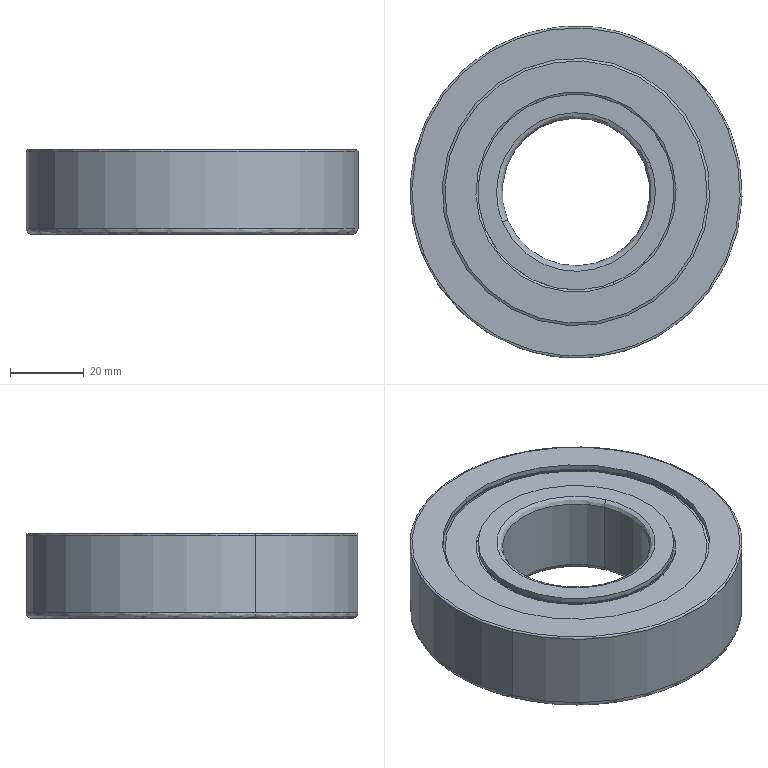Part | SolidWorks | features BaseBody 14 | 14 solids | 277 faces | box 90 x 90 x 23 mm | volume 84067 mm3 | spline 122 | plane 70 | cylinder 65 | cone 20 | commonest cylinder face diameters 72.5 x12 53.125 x8 0.806 x7 1.401 x6 0.999 x5 1.2 x4